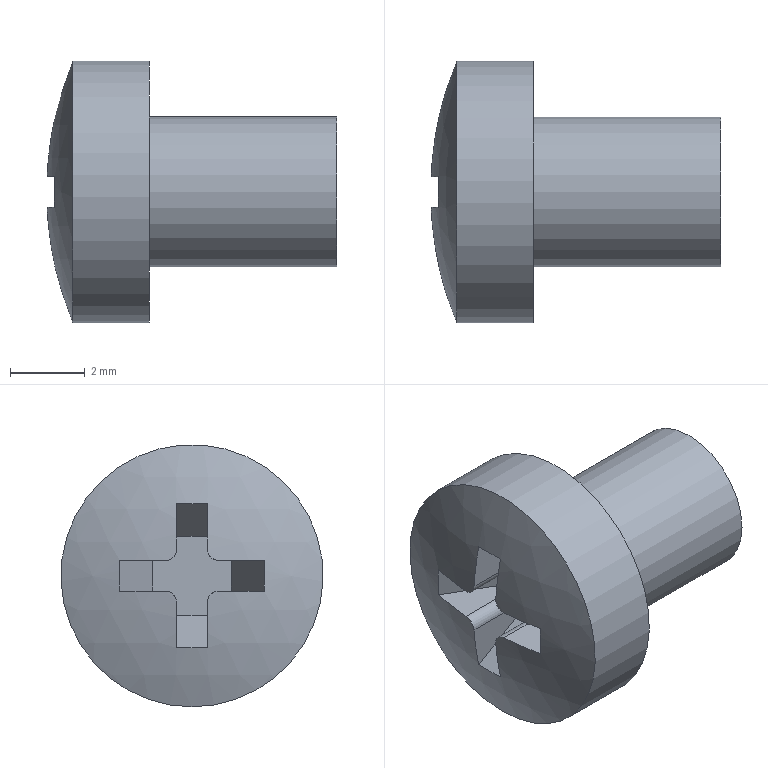Part | STEP file | cross recessed small pan head screws gb_GB_CROSS_SCREWS_TYPE3 M4X5-5-N | 1 solid | 22 faces | box 7.722 x 7 x 7 mm | volume 147.948 mm3 | plane 15 | cylinder 6 | sphere 1 | commonest cylinder face diameters 0.6 x4 4 x1 7 x1